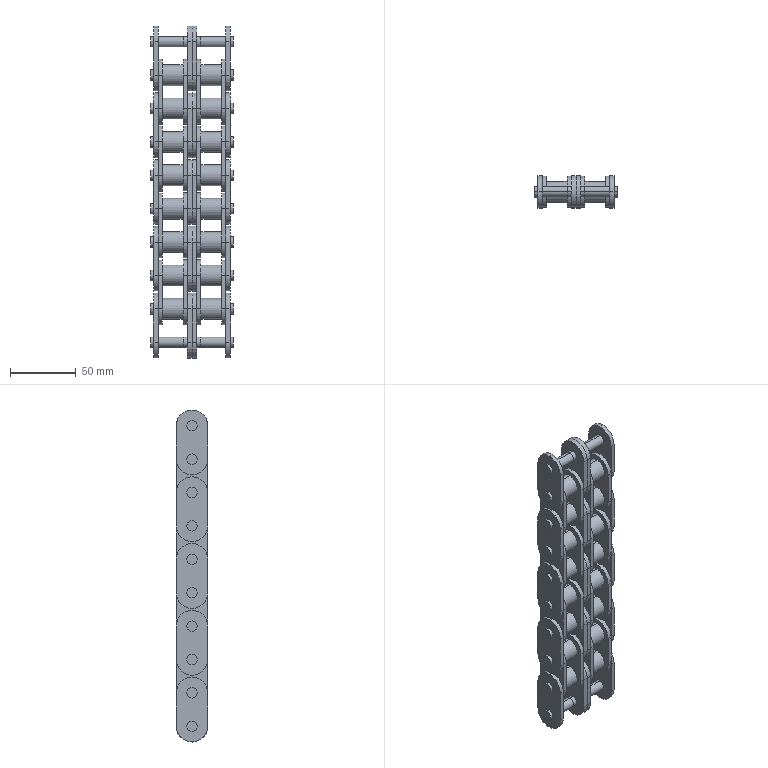Part | SolidWorks | features ICE 7, Extrusion 1, Fillet 1, LPattern 1, MirrorPattern 1, MirrorSolid 1 | 72 solids | 572 faces | box 62.7 x 24 x 252.6 mm | volume 189611 mm3 | cylinder 356 | plane 216 | commonest cylinder face diameters 7.92 x216 24 x108 15.88 x32